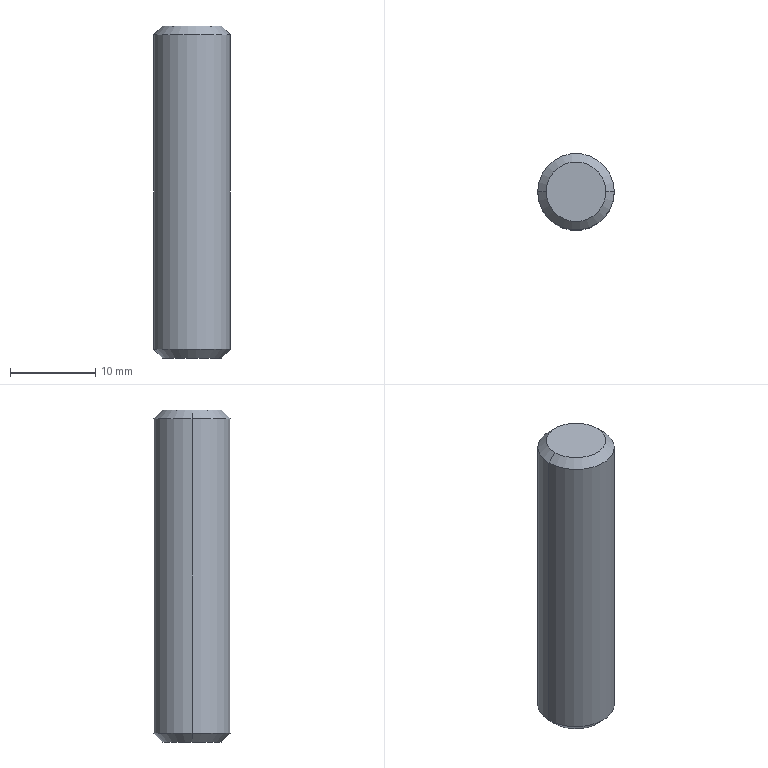Part | SolidWorks | features Chamfer 1, Extrusion 1 | 1 solid | 8 faces | box 9 x 9 x 39 mm | volume 2455 mm3 | cone 4 | cylinder 2 | plane 2 | commonest cylinder face diameters 9 x2
STEP:
#1=CARTESIAN_POINT('',(3.5,0.,39.));
#2=VERTEX_POINT('',#1);
#3=CARTESIAN_POINT('',(-3.5,0.,39.));
#4=VERTEX_POINT('',#3);
#5=CARTESIAN_POINT('',(0.,0.,39.));
#6=DIRECTION('',(0.,0.,1.));
#7=DIRECTION('',(1.,0.,0.));
#8=AXIS2_PLACEMENT_3D('',#5,#6,#7);
#9=CIRCLE('',#8,3.5);
#10=EDGE_CURVE('',#2,#4,#9,.T.);
#11=ORIENTED_EDGE('',*,*,#10,.F.);
#12=CARTESIAN_POINT('',(4.5,0.,38.));
#13=VERTEX_POINT('',#12);
#14=CARTESIAN_POINT('',(3.5,0.,39.));
#15=DIRECTION('',(0.7071,0.,-0.7071));
#16=VECTOR('',#15,1000.);
#17=LINE('',#14,#16);
#18=EDGE_CURVE('',#2,#13,#17,.T.);
#19=ORIENTED_EDGE('',*,*,#18,.T.);
#20=CARTESIAN_POINT('',(-4.5,0.,38.));
#21=VERTEX_POINT('',#20);
#22=CARTESIAN_POINT('',(0.,0.,38.));
#23=DIRECTION('',(0.,0.,-1.));
#24=DIRECTION('',(1.,0.,0.));
#25=AXIS2_PLACEMENT_3D('',#22,#23,#24);
#26=CIRCLE('',#25,4.5);
#27=EDGE_CURVE('',#21,#13,#26,.T.);
#28=ORIENTED_EDGE('',*,*,#27,.F.);
#29=CARTESIAN_POINT('',(-3.5,0.,39.));
#30=DIRECTION('',(-0.7071,0.,-0.7071));
#31=VECTOR('',#30,1000.);
#32=LINE('',#29,#31);
#33=EDGE_CURVE('',#4,#21,#32,.T.);
#34=ORIENTED_EDGE('',*,*,#33,.F.);
#35=EDGE_LOOP('',(#11,#19,#28,#34));
#36=FACE_OUTER_BOUND('',#35,.T.);
#37=CARTESIAN_POINT('',(0.,0.,39.));
#38=DIRECTION('',(0.,0.,-1.));
#39=DIRECTION('',(-1.,0.,0.));
#40=AXIS2_PLACEMENT_3D('',#37,#38,#39);
#41=CONICAL_SURFACE('',#40,3.5,0.7854);
#42=ADVANCED_FACE('',(#36),#41,.T.);
#43=CARTESIAN_POINT('',(-3.5,0.,0.));
#44=VERTEX_POINT('',#43);
#45=CARTESIAN_POINT('',(3.5,0.,0.));
#46=VERTEX_POINT('',#45);
#47=CARTESIAN_POINT('',(0.,0.,0.));
#48=DIRECTION('',(0.,0.,-1.));
#49=DIRECTION('',(1.,0.,0.));
#50=AXIS2_PLACEMENT_3D('',#47,#48,#49);
#51=CIRCLE('',#50,3.5);
#52=EDGE_CURVE('',#44,#46,#51,.T.);
#53=ORIENTED_EDGE('',*,*,#52,.F.);
#54=CARTESIAN_POINT('',(-4.5,0.,1.));
#55=VERTEX_POINT('',#54);
#56=CARTESIAN_POINT('',(-4.5,0.,1.));
#57=DIRECTION('',(-0.7071,0.,0.7071));
#58=VECTOR('',#57,1000.);
#59=LINE('',#56,#58);
#60=EDGE_CURVE('',#44,#55,#59,.T.);
#61=ORIENTED_EDGE('',*,*,#60,.T.);
#62=CARTESIAN_POINT('',(4.5,0.,1.));
#63=VERTEX_POINT('',#62);
#64=CARTESIAN_POINT('',(0.,0.,1.));
#65=DIRECTION('',(0.,0.,1.));
#66=DIRECTION('',(1.,0.,0.));
#67=AXIS2_PLACEMENT_3D('',#64,#65,#66);
#68=CIRCLE('',#67,4.5);
#69=EDGE_CURVE('',#63,#55,#68,.T.);
#70=ORIENTED_EDGE('',*,*,#69,.F.);
#71=CARTESIAN_POINT('',(4.5,0.,1.));
#72=DIRECTION('',(0.7071,0.,0.7071));
#73=VECTOR('',#72,1000.);
#74=LINE('',#71,#73);
#75=EDGE_CURVE('',#46,#63,#74,.T.);
#76=ORIENTED_EDGE('',*,*,#75,.F.);
#77=EDGE_LOOP('',(#53,#61,#70,#76));
#78=FACE_OUTER_BOUND('',#77,.T.);
#79=CARTESIAN_POINT('',(0.,0.,1.));
#80=DIRECTION('',(0.,0.,1.));
#81=DIRECTION('',(1.,0.,0.));
#82=AXIS2_PLACEMENT_3D('',#79,#80,#81);
#83=CONICAL_SURFACE('',#82,4.5,0.7854);
#84=ADVANCED_FACE('',(#78),#83,.T.);
#85=ORIENTED_EDGE('',*,*,#27,.T.);
#86=CARTESIAN_POINT('',(4.5,0.,39.));
#87=DIRECTION('',(0.,0.,-1.));
#88=VECTOR('',#87,1000.);
#89=LINE('',#86,#88);
#90=EDGE_CURVE('',#13,#63,#89,.T.);
#91=ORIENTED_EDGE('',*,*,#90,.T.);
#92=ORIENTED_EDGE('',*,*,#69,.T.);
#93=CARTESIAN_POINT('',(-4.5,0.,39.));
#94=DIRECTION('',(0.,0.,-1.));
#95=VECTOR('',#94,1000.);
#96=LINE('',#93,#95);
#97=EDGE_CURVE('',#21,#55,#96,.T.);
#98=ORIENTED_EDGE('',*,*,#97,.F.);
#99=EDGE_LOOP('',(#85,#91,#92,#98));
#100=FACE_OUTER_BOUND('',#99,.T.);
#101=CARTESIAN_POINT('',(0.,0.,39.));
#102=DIRECTION('',(0.,0.,-1.));
#103=DIRECTION('',(-1.,0.,0.));
#104=AXIS2_PLACEMENT_3D('',#101,#102,#103);
#105=CYLINDRICAL_SURFACE('',#104,4.5);
#106=ADVANCED_FACE('',(#100),#105,.T.);
#107=ORIENTED_EDGE('',*,*,#90,.F.);
#108=CARTESIAN_POINT('',(0.,0.,38.));
#109=DIRECTION('',(0.,0.,-1.));
#110=DIRECTION('',(1.,0.,0.));
#111=AXIS2_PLACEMENT_3D('',#108,#109,#110);
#112=CIRCLE('',#111,4.5);
#113=EDGE_CURVE('',#13,#21,#112,.T.);
#114=ORIENTED_EDGE('',*,*,#113,.T.);
#115=ORIENTED_EDGE('',*,*,#97,.T.);
#116=CARTESIAN_POINT('',(0.,0.,1.));
#117=DIRECTION('',(0.,0.,1.));
#118=DIRECTION('',(1.,0.,0.));
#119=AXIS2_PLACEMENT_3D('',#116,#117,#118);
#120=CIRCLE('',#119,4.5);
#121=EDGE_CURVE('',#55,#63,#120,.T.);
#122=ORIENTED_EDGE('',*,*,#121,.T.);
#123=EDGE_LOOP('',(#107,#114,#115,#122));
#124=FACE_OUTER_BOUND('',#123,.T.);
#125=CARTESIAN_POINT('',(0.,0.,39.));
#126=DIRECTION('',(0.,0.,-1.));
#127=DIRECTION('',(-1.,0.,0.));
#128=AXIS2_PLACEMENT_3D('',#125,#126,#127);
#129=CYLINDRICAL_SURFACE('',#128,4.5);
#130=ADVANCED_FACE('',(#124),#129,.T.);
#131=CARTESIAN_POINT('',(0.,0.,39.));
#132=DIRECTION('',(0.,0.,1.));
#133=DIRECTION('',(1.,0.,0.));
#134=AXIS2_PLACEMENT_3D('',#131,#132,#133);
#135=CIRCLE('',#134,3.5);
#136=EDGE_CURVE('',#4,#2,#135,.T.);
#137=ORIENTED_EDGE('',*,*,#136,.T.);
#138=ORIENTED_EDGE('',*,*,#10,.T.);
#139=EDGE_LOOP('',(#137,#138));
#140=FACE_OUTER_BOUND('',#139,.T.);
#141=CARTESIAN_POINT('',(0.,0.,39.));
#142=DIRECTION('',(0.,0.,1.));
#143=DIRECTION('',(1.,0.,0.));
#144=AXIS2_PLACEMENT_3D('',#141,#142,#143);
#145=PLANE('',#144);
#146=ADVANCED_FACE('',(#140),#145,.T.);
#147=CARTESIAN_POINT('',(0.,0.,0.));
#148=DIRECTION('',(0.,0.,-1.));
#149=DIRECTION('',(1.,0.,0.));
#150=AXIS2_PLACEMENT_3D('',#147,#148,#149);
#151=CIRCLE('',#150,3.5);
#152=EDGE_CURVE('',#46,#44,#151,.T.);
#153=ORIENTED_EDGE('',*,*,#152,.T.);
#154=ORIENTED_EDGE('',*,*,#52,.T.);
#155=EDGE_LOOP('',(#153,#154));
#156=FACE_OUTER_BOUND('',#155,.T.);
#157=CARTESIAN_POINT('',(0.,0.,0.));
#158=DIRECTION('',(0.,0.,1.));
#159=DIRECTION('',(1.,0.,0.));
#160=AXIS2_PLACEMENT_3D('',#157,#158,#159);
#161=PLANE('',#160);
#162=ADVANCED_FACE('',(#156),#161,.F.);
#163=ORIENTED_EDGE('',*,*,#60,.F.);
#164=ORIENTED_EDGE('',*,*,#152,.F.);
#165=ORIENTED_EDGE('',*,*,#75,.T.);
#166=ORIENTED_EDGE('',*,*,#121,.F.);
#167=EDGE_LOOP('',(#163,#164,#165,#166));
#168=FACE_OUTER_BOUND('',#167,.T.);
#169=CARTESIAN_POINT('',(0.,0.,1.));
#170=DIRECTION('',(0.,0.,1.));
#171=DIRECTION('',(1.,0.,0.));
#172=AXIS2_PLACEMENT_3D('',#169,#170,#171);
#173=CONICAL_SURFACE('',#172,4.5,0.7854);
#174=ADVANCED_FACE('',(#168),#173,.T.);
#175=ORIENTED_EDGE('',*,*,#18,.F.);
#176=ORIENTED_EDGE('',*,*,#136,.F.);
#177=ORIENTED_EDGE('',*,*,#33,.T.);
#178=ORIENTED_EDGE('',*,*,#113,.F.);
#179=EDGE_LOOP('',(#175,#176,#177,#178));
#180=FACE_OUTER_BOUND('',#179,.T.);
#181=CARTESIAN_POINT('',(0.,0.,39.));
#182=DIRECTION('',(0.,0.,-1.));
#183=DIRECTION('',(-1.,0.,0.));
#184=AXIS2_PLACEMENT_3D('',#181,#182,#183);
#185=CONICAL_SURFACE('',#184,3.5,0.7854);
#186=ADVANCED_FACE('',(#180),#185,.T.);
#187=CLOSED_SHELL('',(#42,#84,#106,#130,#146,#162,#174,#186));
#188=MANIFOLD_SOLID_BREP('',#187);
#189=CARTESIAN_POINT('',(0.,0.,0.));
#190=DIRECTION('',(0.,0.,1.));
#191=DIRECTION('',(1.,0.,0.));
#192=AXIS2_PLACEMENT_3D('',#189,#190,#191);
#193=(LENGTH_UNIT()NAMED_UNIT(*)SI_UNIT(.MILLI.,.METRE.));
#194=UNCERTAINTY_MEASURE_WITH_UNIT(LENGTH_MEASURE(0.00001),#193,'','');
#195=(NAMED_UNIT(*)PLANE_ANGLE_UNIT()SI_UNIT($,.RADIAN.));
#196=(NAMED_UNIT(*)SI_UNIT($,.STERADIAN.)SOLID_ANGLE_UNIT());
#197=(GEOMETRIC_REPRESENTATION_CONTEXT(3)GLOBAL_UNCERTAINTY_ASSIGNED_CONTEXT((#194))GLOBAL_UNIT_ASSIGNED_CONTEXT((#193,#195,#196))REPRESENTATION_CONTEXT('',''));
#198=ADVANCED_BREP_SHAPE_REPRESENTATION('',(#188,#192),#197);